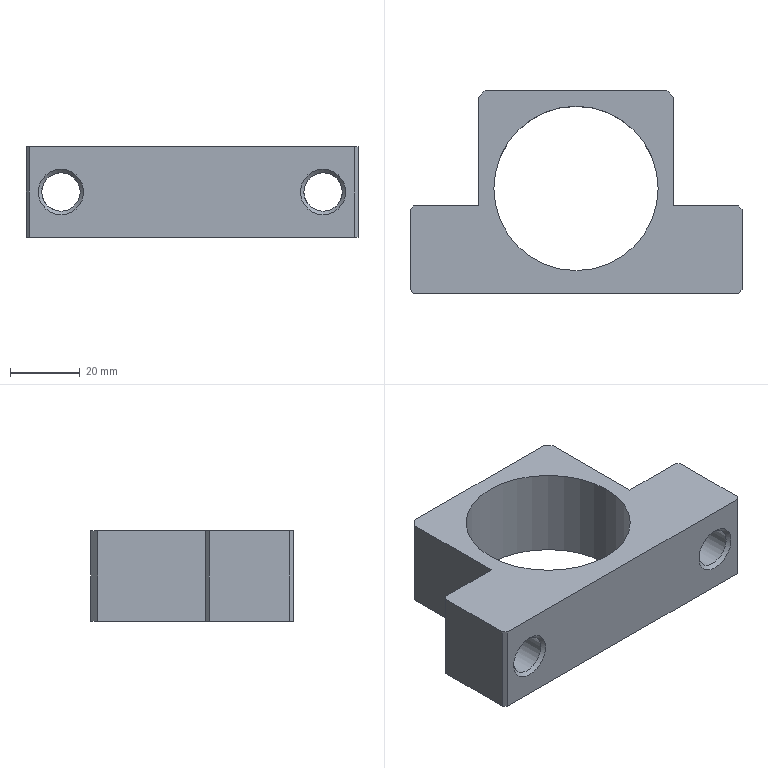Part | NX | 1 solid | 23 faces | box 95 x 58 x 26 mm | volume 59708 mm3 | plane 16 | cone 4 | cylinder 3 | commonest cylinder face diameters 11 x2 47 x1
STEP:
#1=CARTESIAN_POINT('',(-23.5,0.,0.));
#2=VERTEX_POINT('',#1);
#3=CARTESIAN_POINT('',(0.,0.,0.));
#4=DIRECTION('',(0.,0.,-1.));
#5=DIRECTION('',(-1.,0.,0.));
#6=AXIS2_PLACEMENT_3D('',#3,#4,#5);
#7=CIRCLE('',#6,23.5);
#8=EDGE_CURVE('',#2,#2,#7,.F.);
#9=ORIENTED_EDGE('',*,*,#8,.T.);
#10=EDGE_LOOP('',(#9));
#11=FACE_BOUND('',#10,.T.);
#12=CARTESIAN_POINT('',(-23.5,0.,-26.));
#13=VERTEX_POINT('',#12);
#14=CARTESIAN_POINT('',(0.,0.,-26.));
#15=DIRECTION('',(0.,0.,-1.));
#16=DIRECTION('',(-1.,0.,0.));
#17=AXIS2_PLACEMENT_3D('',#14,#15,#16);
#18=CIRCLE('',#17,23.5);
#19=EDGE_CURVE('',#13,#13,#18,.T.);
#20=ORIENTED_EDGE('',*,*,#19,.T.);
#21=EDGE_LOOP('',(#20));
#22=FACE_BOUND('',#21,.T.);
#23=CARTESIAN_POINT('',(0.,0.,0.));
#24=DIRECTION('',(0.,0.,-1.));
#25=DIRECTION('',(-1.,0.,0.));
#26=AXIS2_PLACEMENT_3D('',#23,#24,#25);
#27=CYLINDRICAL_SURFACE('',#26,23.5);
#28=ADVANCED_FACE('',(#11,#22),#27,.F.);
#29=ORIENTED_EDGE('',*,*,#19,.F.);
#30=EDGE_LOOP('',(#29));
#31=FACE_BOUND('',#30,.T.);
#32=CARTESIAN_POINT('',(47.5,-6.,-26.));
#33=VERTEX_POINT('',#32);
#34=CARTESIAN_POINT('',(47.5,-29.,-26.));
#35=VERTEX_POINT('',#34);
#36=CARTESIAN_POINT('',(47.5,-30.,-26.));
#37=DIRECTION('',(0.,1.,0.));
#38=VECTOR('',#37,1000.);
#39=LINE('',#36,#38);
#40=EDGE_CURVE('',#33,#35,#39,.F.);
#41=ORIENTED_EDGE('',*,*,#40,.T.);
#42=CARTESIAN_POINT('',(46.5,-30.,-26.));
#43=VERTEX_POINT('',#42);
#44=CARTESIAN_POINT('',(47.,-29.5,-26.));
#45=DIRECTION('',(0.7071,0.7071,0.));
#46=VECTOR('',#45,1000.);
#47=LINE('',#44,#46);
#48=EDGE_CURVE('',#43,#35,#47,.T.);
#49=ORIENTED_EDGE('',*,*,#48,.F.);
#50=CARTESIAN_POINT('',(-46.5,-30.,-26.));
#51=VERTEX_POINT('',#50);
#52=CARTESIAN_POINT('',(0.,-30.,-26.));
#53=DIRECTION('',(-1.,0.,0.));
#54=VECTOR('',#53,1000.);
#55=LINE('',#52,#54);
#56=EDGE_CURVE('',#43,#51,#55,.T.);
#57=ORIENTED_EDGE('',*,*,#56,.T.);
#58=CARTESIAN_POINT('',(-47.5,-29.,-26.));
#59=VERTEX_POINT('',#58);
#60=CARTESIAN_POINT('',(-47.,-29.5,-26.));
#61=DIRECTION('',(0.7071,-0.7071,0.));
#62=VECTOR('',#61,1000.);
#63=LINE('',#60,#62);
#64=EDGE_CURVE('',#59,#51,#63,.T.);
#65=ORIENTED_EDGE('',*,*,#64,.F.);
#66=CARTESIAN_POINT('',(-47.5,-6.,-26.));
#67=VERTEX_POINT('',#66);
#68=CARTESIAN_POINT('',(-47.5,-30.,-26.));
#69=DIRECTION('',(0.,1.,0.));
#70=VECTOR('',#69,1000.);
#71=LINE('',#68,#70);
#72=EDGE_CURVE('',#59,#67,#71,.T.);
#73=ORIENTED_EDGE('',*,*,#72,.T.);
#74=CARTESIAN_POINT('',(-46.5,-5.,-26.));
#75=VERTEX_POINT('',#74);
#76=CARTESIAN_POINT('',(-47.,-5.5,-26.));
#77=DIRECTION('',(-0.7071,-0.7071,0.));
#78=VECTOR('',#77,1000.);
#79=LINE('',#76,#78);
#80=EDGE_CURVE('',#75,#67,#79,.T.);
#81=ORIENTED_EDGE('',*,*,#80,.F.);
#82=CARTESIAN_POINT('',(-28.,-5.,-26.));
#83=VERTEX_POINT('',#82);
#84=CARTESIAN_POINT('',(0.,-5.,-26.));
#85=DIRECTION('',(1.,0.,0.));
#86=VECTOR('',#85,1000.);
#87=LINE('',#84,#86);
#88=EDGE_CURVE('',#75,#83,#87,.T.);
#89=ORIENTED_EDGE('',*,*,#88,.T.);
#90=CARTESIAN_POINT('',(-28.,26.,-26.));
#91=VERTEX_POINT('',#90);
#92=CARTESIAN_POINT('',(-28.,-30.,-26.));
#93=DIRECTION('',(0.,1.,0.));
#94=VECTOR('',#93,1000.);
#95=LINE('',#92,#94);
#96=EDGE_CURVE('',#83,#91,#95,.T.);
#97=ORIENTED_EDGE('',*,*,#96,.T.);
#98=CARTESIAN_POINT('',(-26.,28.,-26.));
#99=VERTEX_POINT('',#98);
#100=CARTESIAN_POINT('',(-28.,26.,-26.));
#101=CARTESIAN_POINT('',(-27.333,26.667,-26.));
#102=CARTESIAN_POINT('',(-26.667,27.333,-26.));
#103=CARTESIAN_POINT('',(-26.,28.,-26.));
#104=B_SPLINE_CURVE_WITH_KNOTS('',3,(#100,#101,#102,#103),.UNSPECIFIED.,.F.,.F.,(4,4),(0.,1.),.UNSPECIFIED.);
#105=EDGE_CURVE('',#91,#99,#104,.T.);
#106=ORIENTED_EDGE('',*,*,#105,.T.);
#107=CARTESIAN_POINT('',(26.,28.,-26.));
#108=VERTEX_POINT('',#107);
#109=CARTESIAN_POINT('',(0.,28.,-26.));
#110=DIRECTION('',(1.,0.,0.));
#111=VECTOR('',#110,1000.);
#112=LINE('',#109,#111);
#113=EDGE_CURVE('',#99,#108,#112,.T.);
#114=ORIENTED_EDGE('',*,*,#113,.T.);
#115=CARTESIAN_POINT('',(28.,26.,-26.));
#116=VERTEX_POINT('',#115);
#117=CARTESIAN_POINT('',(26.,28.,-26.));
#118=CARTESIAN_POINT('',(26.667,27.333,-26.));
#119=CARTESIAN_POINT('',(27.333,26.667,-26.));
#120=CARTESIAN_POINT('',(28.,26.,-26.));
#121=B_SPLINE_CURVE_WITH_KNOTS('',3,(#117,#118,#119,#120),.UNSPECIFIED.,.F.,.F.,(4,4),(0.,1.),.UNSPECIFIED.);
#122=EDGE_CURVE('',#108,#116,#121,.T.);
#123=ORIENTED_EDGE('',*,*,#122,.T.);
#124=CARTESIAN_POINT('',(28.,-5.,-26.));
#125=VERTEX_POINT('',#124);
#126=CARTESIAN_POINT('',(28.,-30.,-26.));
#127=DIRECTION('',(0.,1.,0.));
#128=VECTOR('',#127,1000.);
#129=LINE('',#126,#128);
#130=EDGE_CURVE('',#116,#125,#129,.F.);
#131=ORIENTED_EDGE('',*,*,#130,.T.);
#132=CARTESIAN_POINT('',(46.5,-5.,-26.));
#133=VERTEX_POINT('',#132);
#134=CARTESIAN_POINT('',(0.,-5.,-26.));
#135=DIRECTION('',(1.,0.,0.));
#136=VECTOR('',#135,1000.);
#137=LINE('',#134,#136);
#138=EDGE_CURVE('',#125,#133,#137,.T.);
#139=ORIENTED_EDGE('',*,*,#138,.T.);
#140=CARTESIAN_POINT('',(47.,-5.5,-26.));
#141=DIRECTION('',(-0.7071,0.7071,0.));
#142=VECTOR('',#141,1000.);
#143=LINE('',#140,#142);
#144=EDGE_CURVE('',#33,#133,#143,.T.);
#145=ORIENTED_EDGE('',*,*,#144,.F.);
#146=EDGE_LOOP('',(#41,#49,#57,#65,#73,#81,#89,#97,#106,#114,#123,#131,#139,#145));
#147=FACE_BOUND('',#146,.T.);
#148=CARTESIAN_POINT('',(47.5,-30.,-26.));
#149=DIRECTION('',(0.,0.,-1.));
#150=DIRECTION('',(-1.,0.,0.));
#151=AXIS2_PLACEMENT_3D('',#148,#149,#150);
#152=PLANE('',#151);
#153=ADVANCED_FACE('',(#31,#147),#152,.T.);
#154=ORIENTED_EDGE('',*,*,#8,.F.);
#155=EDGE_LOOP('',(#154));
#156=FACE_BOUND('',#155,.T.);
#157=CARTESIAN_POINT('',(-47.5,-6.,0.));
#158=VERTEX_POINT('',#157);
#159=CARTESIAN_POINT('',(-46.5,-5.,0.));
#160=VERTEX_POINT('',#159);
#161=CARTESIAN_POINT('',(-47.,-5.5,0.));
#162=DIRECTION('',(0.7071,0.7071,0.));
#163=VECTOR('',#162,1000.);
#164=LINE('',#161,#163);
#165=EDGE_CURVE('',#158,#160,#164,.T.);
#166=ORIENTED_EDGE('',*,*,#165,.F.);
#167=CARTESIAN_POINT('',(-47.5,-29.,0.));
#168=VERTEX_POINT('',#167);
#169=CARTESIAN_POINT('',(-47.5,-30.,0.));
#170=DIRECTION('',(0.,1.,0.));
#171=VECTOR('',#170,1000.);
#172=LINE('',#169,#171);
#173=EDGE_CURVE('',#158,#168,#172,.F.);
#174=ORIENTED_EDGE('',*,*,#173,.T.);
#175=CARTESIAN_POINT('',(-46.5,-30.,0.));
#176=VERTEX_POINT('',#175);
#177=CARTESIAN_POINT('',(-47.,-29.5,0.));
#178=DIRECTION('',(-0.7071,0.7071,0.));
#179=VECTOR('',#178,1000.);
#180=LINE('',#177,#179);
#181=EDGE_CURVE('',#176,#168,#180,.T.);
#182=ORIENTED_EDGE('',*,*,#181,.F.);
#183=CARTESIAN_POINT('',(46.5,-30.,0.));
#184=VERTEX_POINT('',#183);
#185=CARTESIAN_POINT('',(0.,-30.,0.));
#186=DIRECTION('',(1.,0.,0.));
#187=VECTOR('',#186,1000.);
#188=LINE('',#185,#187);
#189=EDGE_CURVE('',#176,#184,#188,.T.);
#190=ORIENTED_EDGE('',*,*,#189,.T.);
#191=CARTESIAN_POINT('',(47.5,-29.,0.));
#192=VERTEX_POINT('',#191);
#193=CARTESIAN_POINT('',(47.,-29.5,0.));
#194=DIRECTION('',(-0.7071,-0.7071,0.));
#195=VECTOR('',#194,1000.);
#196=LINE('',#193,#195);
#197=EDGE_CURVE('',#192,#184,#196,.T.);
#198=ORIENTED_EDGE('',*,*,#197,.F.);
#199=CARTESIAN_POINT('',(47.5,-6.,0.));
#200=VERTEX_POINT('',#199);
#201=CARTESIAN_POINT('',(47.5,-30.,0.));
#202=DIRECTION('',(0.,1.,0.));
#203=VECTOR('',#202,1000.);
#204=LINE('',#201,#203);
#205=EDGE_CURVE('',#192,#200,#204,.T.);
#206=ORIENTED_EDGE('',*,*,#205,.T.);
#207=CARTESIAN_POINT('',(46.5,-5.,0.));
#208=VERTEX_POINT('',#207);
#209=CARTESIAN_POINT('',(47.,-5.5,0.));
#210=DIRECTION('',(0.7071,-0.7071,0.));
#211=VECTOR('',#210,1000.);
#212=LINE('',#209,#211);
#213=EDGE_CURVE('',#208,#200,#212,.T.);
#214=ORIENTED_EDGE('',*,*,#213,.F.);
#215=CARTESIAN_POINT('',(28.,-5.,0.));
#216=VERTEX_POINT('',#215);
#217=CARTESIAN_POINT('',(0.,-5.,0.));
#218=DIRECTION('',(-1.,0.,0.));
#219=VECTOR('',#218,1000.);
#220=LINE('',#217,#219);
#221=EDGE_CURVE('',#208,#216,#220,.T.);
#222=ORIENTED_EDGE('',*,*,#221,.T.);
#223=CARTESIAN_POINT('',(28.,26.,0.));
#224=VERTEX_POINT('',#223);
#225=CARTESIAN_POINT('',(28.,-30.,0.));
#226=DIRECTION('',(0.,1.,0.));
#227=VECTOR('',#226,1000.);
#228=LINE('',#225,#227);
#229=EDGE_CURVE('',#216,#224,#228,.T.);
#230=ORIENTED_EDGE('',*,*,#229,.T.);
#231=CARTESIAN_POINT('',(26.,28.,0.));
#232=VERTEX_POINT('',#231);
#233=CARTESIAN_POINT('',(28.,26.,0.));
#234=CARTESIAN_POINT('',(27.333,26.667,0.));
#235=CARTESIAN_POINT('',(26.667,27.333,0.));
#236=CARTESIAN_POINT('',(26.,28.,0.));
#237=B_SPLINE_CURVE_WITH_KNOTS('',3,(#233,#234,#235,#236),.UNSPECIFIED.,.F.,.F.,(4,4),(0.,1.),.UNSPECIFIED.);
#238=EDGE_CURVE('',#224,#232,#237,.T.);
#239=ORIENTED_EDGE('',*,*,#238,.T.);
#240=CARTESIAN_POINT('',(-26.,28.,0.));
#241=VERTEX_POINT('',#240);
#242=CARTESIAN_POINT('',(0.,28.,0.));
#243=DIRECTION('',(-1.,0.,0.));
#244=VECTOR('',#243,1000.);
#245=LINE('',#242,#244);
#246=EDGE_CURVE('',#232,#241,#245,.T.);
#247=ORIENTED_EDGE('',*,*,#246,.T.);
#248=CARTESIAN_POINT('',(-28.,26.,0.));
#249=VERTEX_POINT('',#248);
#250=CARTESIAN_POINT('',(-26.,28.,0.));
#251=CARTESIAN_POINT('',(-26.667,27.333,0.));
#252=CARTESIAN_POINT('',(-27.333,26.667,0.));
#253=CARTESIAN_POINT('',(-28.,26.,0.));
#254=B_SPLINE_CURVE_WITH_KNOTS('',3,(#250,#251,#252,#253),.UNSPECIFIED.,.F.,.F.,(4,4),(0.,1.),.UNSPECIFIED.);
#255=EDGE_CURVE('',#241,#249,#254,.T.);
#256=ORIENTED_EDGE('',*,*,#255,.T.);
#257=CARTESIAN_POINT('',(-28.,-5.,0.));
#258=VERTEX_POINT('',#257);
#259=CARTESIAN_POINT('',(-28.,-30.,0.));
#260=DIRECTION('',(0.,1.,0.));
#261=VECTOR('',#260,1000.);
#262=LINE('',#259,#261);
#263=EDGE_CURVE('',#249,#258,#262,.F.);
#264=ORIENTED_EDGE('',*,*,#263,.T.);
#265=CARTESIAN_POINT('',(0.,-5.,0.));
#266=DIRECTION('',(-1.,0.,0.));
#267=VECTOR('',#266,1000.);
#268=LINE('',#265,#267);
#269=EDGE_CURVE('',#258,#160,#268,.T.);
#270=ORIENTED_EDGE('',*,*,#269,.T.);
#271=EDGE_LOOP('',(#166,#174,#182,#190,#198,#206,#214,#222,#230,#239,#247,#256,#264,#270));
#272=FACE_BOUND('',#271,.T.);
#273=CARTESIAN_POINT('',(-47.5,-30.,0.));
#274=DIRECTION('',(0.,0.,1.));
#275=DIRECTION('',(1.,0.,0.));
#276=AXIS2_PLACEMENT_3D('',#273,#274,#275);
#277=PLANE('',#276);
#278=ADVANCED_FACE('',(#156,#272),#277,.T.);
#279=ORIENTED_EDGE('',*,*,#205,.F.);
#280=CARTESIAN_POINT('',(47.5,-29.,0.));
#281=DIRECTION('',(0.,0.,-1.));
#282=VECTOR('',#281,1000.);
#283=LINE('',#280,#282);
#284=EDGE_CURVE('',#192,#35,#283,.T.);
#285=ORIENTED_EDGE('',*,*,#284,.T.);
#286=ORIENTED_EDGE('',*,*,#40,.F.);
#287=CARTESIAN_POINT('',(47.5,-6.,0.));
#288=DIRECTION('',(0.,0.,-1.));
#289=VECTOR('',#288,1000.);
#290=LINE('',#287,#289);
#291=EDGE_CURVE('',#33,#200,#290,.F.);
#292=ORIENTED_EDGE('',*,*,#291,.T.);
#293=EDGE_LOOP('',(#279,#285,#286,#292));
#294=FACE_BOUND('',#293,.T.);
#295=CARTESIAN_POINT('',(47.5,-6.,0.));
#296=DIRECTION('',(1.,0.,0.));
#297=DIRECTION('',(0.,-1.,0.));
#298=AXIS2_PLACEMENT_3D('',#295,#296,#297);
#299=PLANE('',#298);
#300=ADVANCED_FACE('',(#294),#299,.T.);
#301=CARTESIAN_POINT('',(37.5,-5.,-6.5));
#302=VERTEX_POINT('',#301);
#303=CARTESIAN_POINT('',(37.5,-5.,-13.));
#304=DIRECTION('',(0.,1.,0.));
#305=DIRECTION('',(0.,0.,1.));
#306=AXIS2_PLACEMENT_3D('',#303,#304,#305);
#307=CIRCLE('',#306,6.5);
#308=EDGE_CURVE('',#302,#302,#307,.F.);
#309=ORIENTED_EDGE('',*,*,#308,.T.);
#310=EDGE_LOOP('',(#309));
#311=FACE_BOUND('',#310,.T.);
#312=ORIENTED_EDGE('',*,*,#221,.F.);
#313=CARTESIAN_POINT('',(46.5,-5.,0.));
#314=DIRECTION('',(0.,0.,-1.));
#315=VECTOR('',#314,1000.);
#316=LINE('',#313,#315);
#317=EDGE_CURVE('',#208,#133,#316,.T.);
#318=ORIENTED_EDGE('',*,*,#317,.T.);
#319=ORIENTED_EDGE('',*,*,#138,.F.);
#320=CARTESIAN_POINT('',(28.,-5.,0.));
#321=DIRECTION('',(0.,0.,-1.));
#322=VECTOR('',#321,1000.);
#323=LINE('',#320,#322);
#324=EDGE_CURVE('',#125,#216,#323,.F.);
#325=ORIENTED_EDGE('',*,*,#324,.T.);
#326=EDGE_LOOP('',(#312,#318,#319,#325));
#327=FACE_BOUND('',#326,.T.);
#328=CARTESIAN_POINT('',(28.,-5.,0.));
#329=DIRECTION('',(0.,1.,0.));
#330=DIRECTION('',(1.,0.,0.));
#331=AXIS2_PLACEMENT_3D('',#328,#329,#330);
#332=PLANE('',#331);
#333=ADVANCED_FACE('',(#311,#327),#332,.T.);
#334=ORIENTED_EDGE('',*,*,#229,.F.);
#335=ORIENTED_EDGE('',*,*,#324,.F.);
#336=ORIENTED_EDGE('',*,*,#130,.F.);
#337=CARTESIAN_POINT('',(28.,26.,0.));
#338=DIRECTION('',(0.,0.,-1.));
#339=VECTOR('',#338,1000.);
#340=LINE('',#337,#339);
#341=EDGE_CURVE('',#116,#224,#340,.F.);
#342=ORIENTED_EDGE('',*,*,#341,.T.);
#343=EDGE_LOOP('',(#334,#335,#336,#342));
#344=FACE_BOUND('',#343,.T.);
#345=CARTESIAN_POINT('',(28.,26.,0.));
#346=DIRECTION('',(1.,0.,0.));
#347=DIRECTION('',(0.,-1.,0.));
#348=AXIS2_PLACEMENT_3D('',#345,#346,#347);
#349=PLANE('',#348);
#350=ADVANCED_FACE('',(#344),#349,.T.);
#351=ORIENTED_EDGE('',*,*,#238,.F.);
#352=ORIENTED_EDGE('',*,*,#341,.F.);
#353=ORIENTED_EDGE('',*,*,#122,.F.);
#354=CARTESIAN_POINT('',(26.,28.,0.));
#355=DIRECTION('',(0.,0.,-1.));
#356=VECTOR('',#355,1000.);
#357=LINE('',#354,#356);
#358=EDGE_CURVE('',#108,#232,#357,.F.);
#359=ORIENTED_EDGE('',*,*,#358,.T.);
#360=EDGE_LOOP('',(#351,#352,#353,#359));
#361=FACE_BOUND('',#360,.T.);
#362=CARTESIAN_POINT('',(26.,28.,0.));
#363=DIRECTION('',(0.7071,0.7071,0.));
#364=DIRECTION('',(0.7071,-0.7071,0.));
#365=AXIS2_PLACEMENT_3D('',#362,#363,#364);
#366=PLANE('',#365);
#367=ADVANCED_FACE('',(#361),#366,.T.);
#368=ORIENTED_EDGE('',*,*,#246,.F.);
#369=ORIENTED_EDGE('',*,*,#358,.F.);
#370=ORIENTED_EDGE('',*,*,#113,.F.);
#371=CARTESIAN_POINT('',(-26.,28.,0.));
#372=DIRECTION('',(0.,0.,-1.));
#373=VECTOR('',#372,1000.);
#374=LINE('',#371,#373);
#375=EDGE_CURVE('',#99,#241,#374,.F.);
#376=ORIENTED_EDGE('',*,*,#375,.T.);
#377=EDGE_LOOP('',(#368,#369,#370,#376));
#378=FACE_BOUND('',#377,.T.);
#379=CARTESIAN_POINT('',(-26.,28.,0.));
#380=DIRECTION('',(0.,1.,0.));
#381=DIRECTION('',(1.,0.,0.));
#382=AXIS2_PLACEMENT_3D('',#379,#380,#381);
#383=PLANE('',#382);
#384=ADVANCED_FACE('',(#378),#383,.T.);
#385=ORIENTED_EDGE('',*,*,#255,.F.);
#386=ORIENTED_EDGE('',*,*,#375,.F.);
#387=ORIENTED_EDGE('',*,*,#105,.F.);
#388=CARTESIAN_POINT('',(-28.,26.,0.));
#389=DIRECTION('',(0.,0.,-1.));
#390=VECTOR('',#389,1000.);
#391=LINE('',#388,#390);
#392=EDGE_CURVE('',#91,#249,#391,.F.);
#393=ORIENTED_EDGE('',*,*,#392,.T.);
#394=EDGE_LOOP('',(#385,#386,#387,#393));
#395=FACE_BOUND('',#394,.T.);
#396=CARTESIAN_POINT('',(-28.,26.,0.));
#397=DIRECTION('',(-0.7071,0.7071,0.));
#398=DIRECTION('',(0.7071,0.7071,0.));
#399=AXIS2_PLACEMENT_3D('',#396,#397,#398);
#400=PLANE('',#399);
#401=ADVANCED_FACE('',(#395),#400,.T.);
#402=ORIENTED_EDGE('',*,*,#263,.F.);
#403=ORIENTED_EDGE('',*,*,#392,.F.);
#404=ORIENTED_EDGE('',*,*,#96,.F.);
#405=CARTESIAN_POINT('',(-28.,-5.,0.));
#406=DIRECTION('',(0.,0.,-1.));
#407=VECTOR('',#406,1000.);
#408=LINE('',#405,#407);
#409=EDGE_CURVE('',#83,#258,#408,.F.);
#410=ORIENTED_EDGE('',*,*,#409,.T.);
#411=EDGE_LOOP('',(#402,#403,#404,#410));
#412=FACE_BOUND('',#411,.T.);
#413=CARTESIAN_POINT('',(-28.,-5.,0.));
#414=DIRECTION('',(-1.,0.,0.));
#415=DIRECTION('',(0.,1.,0.));
#416=AXIS2_PLACEMENT_3D('',#413,#414,#415);
#417=PLANE('',#416);
#418=ADVANCED_FACE('',(#412),#417,.T.);
#419=CARTESIAN_POINT('',(-37.5,-5.,-6.5));
#420=VERTEX_POINT('',#419);
#421=CARTESIAN_POINT('',(-37.5,-5.,-13.));
#422=DIRECTION('',(0.,1.,0.));
#423=DIRECTION('',(0.,0.,1.));
#424=AXIS2_PLACEMENT_3D('',#421,#422,#423);
#425=CIRCLE('',#424,6.5);
#426=EDGE_CURVE('',#420,#420,#425,.F.);
#427=ORIENTED_EDGE('',*,*,#426,.T.);
#428=EDGE_LOOP('',(#427));
#429=FACE_BOUND('',#428,.T.);
#430=ORIENTED_EDGE('',*,*,#269,.F.);
#431=ORIENTED_EDGE('',*,*,#409,.F.);
#432=ORIENTED_EDGE('',*,*,#88,.F.);
#433=CARTESIAN_POINT('',(-46.5,-5.,0.));
#434=DIRECTION('',(0.,0.,-1.));
#435=VECTOR('',#434,1000.);
#436=LINE('',#433,#435);
#437=EDGE_CURVE('',#75,#160,#436,.F.);
#438=ORIENTED_EDGE('',*,*,#437,.T.);
#439=EDGE_LOOP('',(#430,#431,#432,#438));
#440=FACE_BOUND('',#439,.T.);
#441=CARTESIAN_POINT('',(-46.5,-5.,0.));
#442=DIRECTION('',(0.,1.,0.));
#443=DIRECTION('',(1.,0.,0.));
#444=AXIS2_PLACEMENT_3D('',#441,#442,#443);
#445=PLANE('',#444);
#446=ADVANCED_FACE('',(#429,#440),#445,.T.);
#447=ORIENTED_EDGE('',*,*,#173,.F.);
#448=CARTESIAN_POINT('',(-47.5,-6.,0.));
#449=DIRECTION('',(0.,0.,-1.));
#450=VECTOR('',#449,1000.);
#451=LINE('',#448,#450);
#452=EDGE_CURVE('',#158,#67,#451,.T.);
#453=ORIENTED_EDGE('',*,*,#452,.T.);
#454=ORIENTED_EDGE('',*,*,#72,.F.);
#455=CARTESIAN_POINT('',(-47.5,-29.,0.));
#456=DIRECTION('',(0.,0.,-1.));
#457=VECTOR('',#456,1000.);
#458=LINE('',#455,#457);
#459=EDGE_CURVE('',#59,#168,#458,.F.);
#460=ORIENTED_EDGE('',*,*,#459,.T.);
#461=EDGE_LOOP('',(#447,#453,#454,#460));
#462=FACE_BOUND('',#461,.T.);
#463=CARTESIAN_POINT('',(-47.5,-29.,0.));
#464=DIRECTION('',(-1.,0.,0.));
#465=DIRECTION('',(0.,1.,0.));
#466=AXIS2_PLACEMENT_3D('',#463,#464,#465);
#467=PLANE('',#466);
#468=ADVANCED_FACE('',(#462),#467,.T.);
#469=CARTESIAN_POINT('',(37.5,-30.,-19.5));
#470=VERTEX_POINT('',#469);
#471=CARTESIAN_POINT('',(37.5,-30.,-13.));
#472=DIRECTION('',(0.,-1.,0.));
#473=DIRECTION('',(0.,0.,-1.));
#474=AXIS2_PLACEMENT_3D('',#471,#472,#473);
#475=CIRCLE('',#474,6.5);
#476=EDGE_CURVE('',#470,#470,#475,.F.);
#477=ORIENTED_EDGE('',*,*,#476,.T.);
#478=EDGE_LOOP('',(#477));
#479=FACE_BOUND('',#478,.T.);
#480=CARTESIAN_POINT('',(-37.5,-30.,-19.5));
#481=VERTEX_POINT('',#480);
#482=CARTESIAN_POINT('',(-37.5,-30.,-13.));
#483=DIRECTION('',(0.,-1.,0.));
#484=DIRECTION('',(0.,0.,-1.));
#485=AXIS2_PLACEMENT_3D('',#482,#483,#484);
#486=CIRCLE('',#485,6.5);
#487=EDGE_CURVE('',#481,#481,#486,.F.);
#488=ORIENTED_EDGE('',*,*,#487,.T.);
#489=EDGE_LOOP('',(#488));
#490=FACE_BOUND('',#489,.T.);
#491=ORIENTED_EDGE('',*,*,#189,.F.);
#492=CARTESIAN_POINT('',(-46.5,-30.,0.));
#493=DIRECTION('',(0.,0.,-1.));
#494=VECTOR('',#493,1000.);
#495=LINE('',#492,#494);
#496=EDGE_CURVE('',#176,#51,#495,.T.);
#497=ORIENTED_EDGE('',*,*,#496,.T.);
#498=ORIENTED_EDGE('',*,*,#56,.F.);
#499=CARTESIAN_POINT('',(46.5,-30.,0.));
#500=DIRECTION('',(0.,0.,-1.));
#501=VECTOR('',#500,1000.);
#502=LINE('',#499,#501);
#503=EDGE_CURVE('',#43,#184,#502,.F.);
#504=ORIENTED_EDGE('',*,*,#503,.T.);
#505=EDGE_LOOP('',(#491,#497,#498,#504));
#506=FACE_BOUND('',#505,.T.);
#507=CARTESIAN_POINT('',(46.5,-30.,0.));
#508=DIRECTION('',(0.,-1.,0.));
#509=DIRECTION('',(-1.,0.,0.));
#510=AXIS2_PLACEMENT_3D('',#507,#508,#509);
#511=PLANE('',#510);
#512=ADVANCED_FACE('',(#479,#490,#506),#511,.T.);
#513=ORIENTED_EDGE('',*,*,#197,.T.);
#514=ORIENTED_EDGE('',*,*,#503,.F.);
#515=ORIENTED_EDGE('',*,*,#48,.T.);
#516=ORIENTED_EDGE('',*,*,#284,.F.);
#517=EDGE_LOOP('',(#513,#514,#515,#516));
#518=FACE_BOUND('',#517,.T.);
#519=CARTESIAN_POINT('',(47.5,-29.,0.));
#520=DIRECTION('',(0.7071,-0.7071,0.));
#521=DIRECTION('',(-0.7071,-0.7071,0.));
#522=AXIS2_PLACEMENT_3D('',#519,#520,#521);
#523=PLANE('',#522);
#524=ADVANCED_FACE('',(#518),#523,.T.);
#525=ORIENTED_EDGE('',*,*,#213,.T.);
#526=ORIENTED_EDGE('',*,*,#291,.F.);
#527=ORIENTED_EDGE('',*,*,#144,.T.);
#528=ORIENTED_EDGE('',*,*,#317,.F.);
#529=EDGE_LOOP('',(#525,#526,#527,#528));
#530=FACE_BOUND('',#529,.T.);
#531=CARTESIAN_POINT('',(46.5,-5.,0.));
#532=DIRECTION('',(0.7071,0.7071,0.));
#533=DIRECTION('',(0.7071,-0.7071,0.));
#534=AXIS2_PLACEMENT_3D('',#531,#532,#533);
#535=PLANE('',#534);
#536=ADVANCED_FACE('',(#530),#535,.T.);
#537=ORIENTED_EDGE('',*,*,#308,.F.);
#538=EDGE_LOOP('',(#537));
#539=FACE_BOUND('',#538,.T.);
#540=CARTESIAN_POINT('',(43.,-6.,-13.));
#541=VERTEX_POINT('',#540);
#542=CARTESIAN_POINT('',(37.5,-6.,-13.));
#543=DIRECTION('',(0.,-1.,0.));
#544=DIRECTION('',(1.,0.,0.));
#545=AXIS2_PLACEMENT_3D('',#542,#543,#544);
#546=CIRCLE('',#545,5.5);
#547=EDGE_CURVE('',#541,#541,#546,.T.);
#548=ORIENTED_EDGE('',*,*,#547,.T.);
#549=EDGE_LOOP('',(#548));
#550=FACE_BOUND('',#549,.T.);
#551=CARTESIAN_POINT('',(37.5,-5.,-13.));
#552=DIRECTION('',(0.,1.,0.));
#553=DIRECTION('',(0.,0.,1.));
#554=AXIS2_PLACEMENT_3D('',#551,#552,#553);
#555=CONICAL_SURFACE('',#554,6.5,0.7854);
#556=ADVANCED_FACE('',(#539,#550),#555,.F.);
#557=ORIENTED_EDGE('',*,*,#426,.F.);
#558=EDGE_LOOP('',(#557));
#559=FACE_BOUND('',#558,.T.);
#560=CARTESIAN_POINT('',(-32.,-6.,-13.));
#561=VERTEX_POINT('',#560);
#562=CARTESIAN_POINT('',(-37.5,-6.,-13.));
#563=DIRECTION('',(0.,-1.,0.));
#564=DIRECTION('',(1.,0.,0.));
#565=AXIS2_PLACEMENT_3D('',#562,#563,#564);
#566=CIRCLE('',#565,5.5);
#567=EDGE_CURVE('',#561,#561,#566,.T.);
#568=ORIENTED_EDGE('',*,*,#567,.T.);
#569=EDGE_LOOP('',(#568));
#570=FACE_BOUND('',#569,.T.);
#571=CARTESIAN_POINT('',(-37.5,-5.,-13.));
#572=DIRECTION('',(0.,1.,0.));
#573=DIRECTION('',(0.,0.,1.));
#574=AXIS2_PLACEMENT_3D('',#571,#572,#573);
#575=CONICAL_SURFACE('',#574,6.5,0.7854);
#576=ADVANCED_FACE('',(#559,#570),#575,.F.);
#577=ORIENTED_EDGE('',*,*,#165,.T.);
#578=ORIENTED_EDGE('',*,*,#437,.F.);
#579=ORIENTED_EDGE('',*,*,#80,.T.);
#580=ORIENTED_EDGE('',*,*,#452,.F.);
#581=EDGE_LOOP('',(#577,#578,#579,#580));
#582=FACE_BOUND('',#581,.T.);
#583=CARTESIAN_POINT('',(-47.5,-6.,0.));
#584=DIRECTION('',(-0.7071,0.7071,0.));
#585=DIRECTION('',(0.7071,0.7071,0.));
#586=AXIS2_PLACEMENT_3D('',#583,#584,#585);
#587=PLANE('',#586);
#588=ADVANCED_FACE('',(#582),#587,.T.);
#589=ORIENTED_EDGE('',*,*,#181,.T.);
#590=ORIENTED_EDGE('',*,*,#459,.F.);
#591=ORIENTED_EDGE('',*,*,#64,.T.);
#592=ORIENTED_EDGE('',*,*,#496,.F.);
#593=EDGE_LOOP('',(#589,#590,#591,#592));
#594=FACE_BOUND('',#593,.T.);
#595=CARTESIAN_POINT('',(-46.5,-30.,0.));
#596=DIRECTION('',(-0.7071,-0.7071,0.));
#597=DIRECTION('',(-0.7071,0.7071,0.));
#598=AXIS2_PLACEMENT_3D('',#595,#596,#597);
#599=PLANE('',#598);
#600=ADVANCED_FACE('',(#594),#599,.T.);
#601=ORIENTED_EDGE('',*,*,#476,.F.);
#602=EDGE_LOOP('',(#601));
#603=FACE_BOUND('',#602,.T.);
#604=CARTESIAN_POINT('',(43.,-29.,-13.));
#605=VERTEX_POINT('',#604);
#606=CARTESIAN_POINT('',(37.5,-29.,-13.));
#607=DIRECTION('',(0.,1.,0.));
#608=DIRECTION('',(1.,0.,0.));
#609=AXIS2_PLACEMENT_3D('',#606,#607,#608);
#610=CIRCLE('',#609,5.5);
#611=EDGE_CURVE('',#605,#605,#610,.T.);
#612=ORIENTED_EDGE('',*,*,#611,.T.);
#613=EDGE_LOOP('',(#612));
#614=FACE_BOUND('',#613,.T.);
#615=CARTESIAN_POINT('',(37.5,-30.,-13.));
#616=DIRECTION('',(0.,-1.,0.));
#617=DIRECTION('',(0.,0.,-1.));
#618=AXIS2_PLACEMENT_3D('',#615,#616,#617);
#619=CONICAL_SURFACE('',#618,6.5,0.7854);
#620=ADVANCED_FACE('',(#603,#614),#619,.F.);
#621=ORIENTED_EDGE('',*,*,#487,.F.);
#622=EDGE_LOOP('',(#621));
#623=FACE_BOUND('',#622,.T.);
#624=CARTESIAN_POINT('',(-32.,-29.,-13.));
#625=VERTEX_POINT('',#624);
#626=CARTESIAN_POINT('',(-37.5,-29.,-13.));
#627=DIRECTION('',(0.,1.,0.));
#628=DIRECTION('',(1.,0.,0.));
#629=AXIS2_PLACEMENT_3D('',#626,#627,#628);
#630=CIRCLE('',#629,5.5);
#631=EDGE_CURVE('',#625,#625,#630,.T.);
#632=ORIENTED_EDGE('',*,*,#631,.T.);
#633=EDGE_LOOP('',(#632));
#634=FACE_BOUND('',#633,.T.);
#635=CARTESIAN_POINT('',(-37.5,-30.,-13.));
#636=DIRECTION('',(0.,-1.,0.));
#637=DIRECTION('',(0.,0.,-1.));
#638=AXIS2_PLACEMENT_3D('',#635,#636,#637);
#639=CONICAL_SURFACE('',#638,6.5,0.7854);
#640=ADVANCED_FACE('',(#623,#634),#639,.F.);
#641=ORIENTED_EDGE('',*,*,#547,.F.);
#642=EDGE_LOOP('',(#641));
#643=FACE_BOUND('',#642,.T.);
#644=ORIENTED_EDGE('',*,*,#611,.F.);
#645=EDGE_LOOP('',(#644));
#646=FACE_BOUND('',#645,.T.);
#647=CARTESIAN_POINT('',(37.5,-29.,-13.));
#648=DIRECTION('',(0.,1.,0.));
#649=DIRECTION('',(0.,0.,1.));
#650=AXIS2_PLACEMENT_3D('',#647,#648,#649);
#651=CYLINDRICAL_SURFACE('',#650,5.5);
#652=ADVANCED_FACE('',(#643,#646),#651,.F.);
#653=ORIENTED_EDGE('',*,*,#567,.F.);
#654=EDGE_LOOP('',(#653));
#655=FACE_BOUND('',#654,.T.);
#656=ORIENTED_EDGE('',*,*,#631,.F.);
#657=EDGE_LOOP('',(#656));
#658=FACE_BOUND('',#657,.T.);
#659=CARTESIAN_POINT('',(-37.5,-29.,-13.));
#660=DIRECTION('',(0.,1.,0.));
#661=DIRECTION('',(0.,0.,1.));
#662=AXIS2_PLACEMENT_3D('',#659,#660,#661);
#663=CYLINDRICAL_SURFACE('',#662,5.5);
#664=ADVANCED_FACE('',(#655,#658),#663,.F.);
#665=CLOSED_SHELL('',(#28,#153,#278,#300,#333,#350,#367,#384,#401,#418,#446,#468,#512,#524,#536,#556,#576,#588,#600,#620,#640,#652,#664));
#666=MANIFOLD_SOLID_BREP('',#665);
#667=(LENGTH_UNIT()NAMED_UNIT(*)SI_UNIT(.MILLI.,.METRE.));
#668=UNCERTAINTY_MEASURE_WITH_UNIT(LENGTH_MEASURE(0.0508),#667,'','');
#669=(NAMED_UNIT(*)PLANE_ANGLE_UNIT()SI_UNIT($,.RADIAN.));
#670=(NAMED_UNIT(*)SI_UNIT($,.STERADIAN.)SOLID_ANGLE_UNIT());
#671=(GEOMETRIC_REPRESENTATION_CONTEXT(3)GLOBAL_UNCERTAINTY_ASSIGNED_CONTEXT((#668))GLOBAL_UNIT_ASSIGNED_CONTEXT((#667,#669,#670))REPRESENTATION_CONTEXT('',''));
#672=ADVANCED_BREP_SHAPE_REPRESENTATION('',(#666),#671);